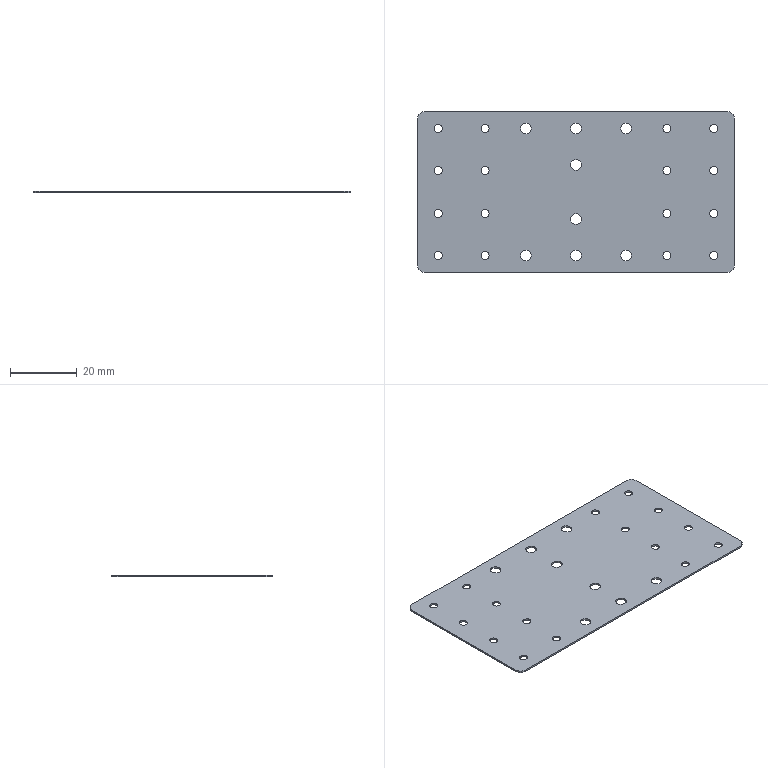Part | SolidWorks | features BaseBody 1 | 1 solid | 58 faces | box 94.8 x 48 x 0.5 mm | volume 2205 mm3 | cylinder 52 | plane 6 | commonest cylinder face diameters 2.4 x32 3.2 x16 4 x4